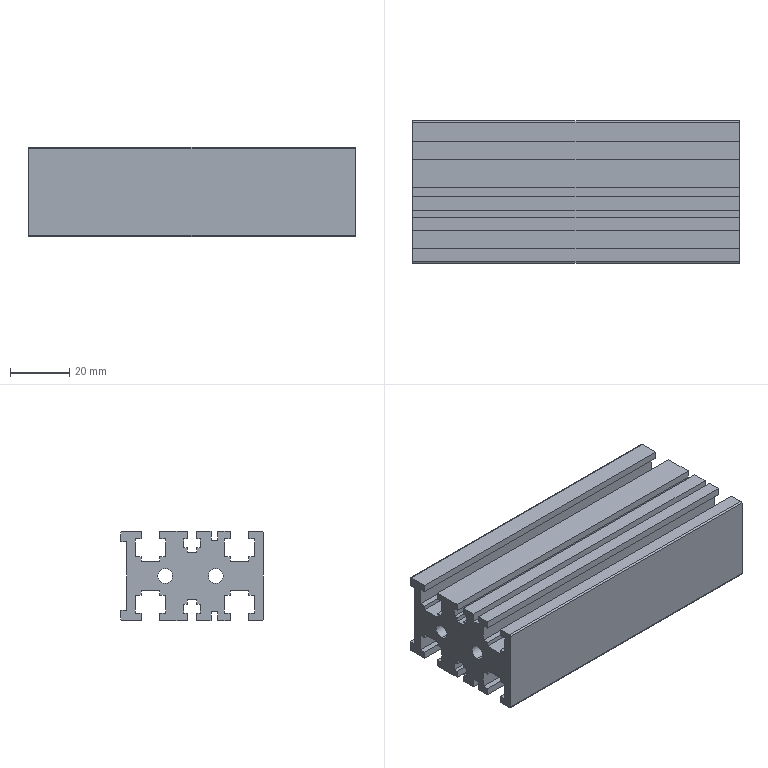Part | STEP file | Guide wheel mechanism revised.sldasm-Part-52 | 1 solid | 98 faces | box 110 x 48 x 30 mm | volume 103127 mm3 | plane 90 | cylinder 8 | commonest cylinder face diameters 1 x4 5 x4